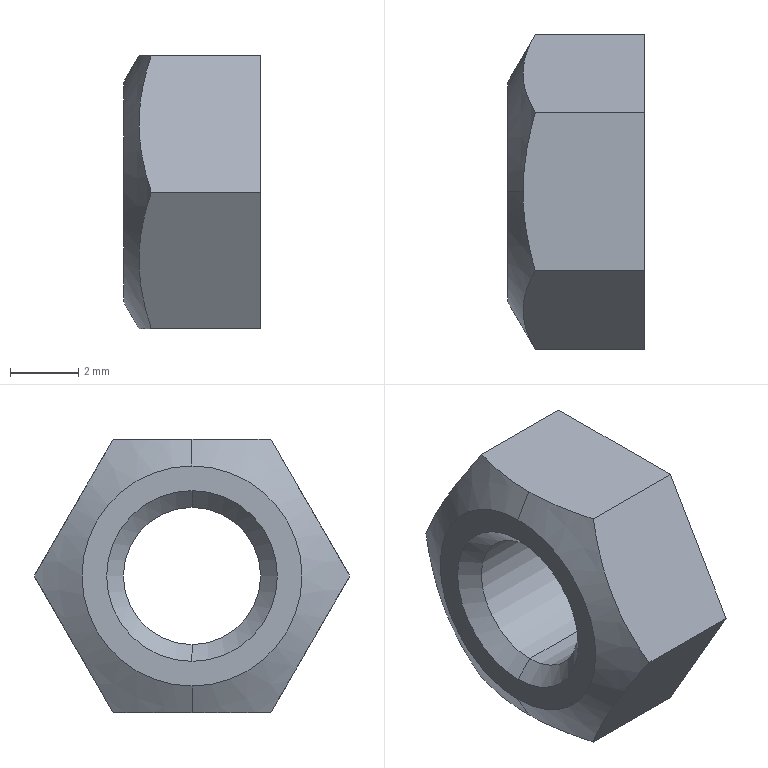Part | SolidWorks | features ICE 1, RevCut 1, Revolution 1 | 1 solid | 16 faces | box 4 x 9.238 x 8 mm | volume 160.7 mm3 | plane 8 | cone 6 | cylinder 2 | commonest cylinder face diameters 4.017 x2
STEP:
#1=CARTESIAN_POINT('',(-0.4915,0.,-2.009));
#2=VERTEX_POINT('',#1);
#3=CARTESIAN_POINT('',(-0.4915,0.,2.009));
#4=VERTEX_POINT('',#3);
#5=CARTESIAN_POINT('',(-0.4915,0.,0.));
#6=DIRECTION('',(-1.,0.,0.));
#7=DIRECTION('',(0.,0.,1.));
#8=AXIS2_PLACEMENT_3D('',#5,#6,#7);
#9=CIRCLE('',#8,2.009);
#10=EDGE_CURVE('',#2,#4,#9,.T.);
#11=ORIENTED_EDGE('',*,*,#10,.T.);
#12=CARTESIAN_POINT('',(0.,0.,2.5));
#13=VERTEX_POINT('',#12);
#14=CARTESIAN_POINT('',(0.,0.,2.5));
#15=DIRECTION('',(0.7071,0.,0.7071));
#16=VECTOR('',#15,1000.);
#17=LINE('',#14,#16);
#18=EDGE_CURVE('',#4,#13,#17,.T.);
#19=ORIENTED_EDGE('',*,*,#18,.T.);
#20=CARTESIAN_POINT('',(0.,0.,-2.5));
#21=VERTEX_POINT('',#20);
#22=CARTESIAN_POINT('',(0.,0.,0.));
#23=DIRECTION('',(-1.,0.,0.));
#24=DIRECTION('',(0.,0.,1.));
#25=AXIS2_PLACEMENT_3D('',#22,#23,#24);
#26=CIRCLE('',#25,2.5);
#27=EDGE_CURVE('',#21,#13,#26,.T.);
#28=ORIENTED_EDGE('',*,*,#27,.F.);
#29=CARTESIAN_POINT('',(0.,0.,-2.5));
#30=DIRECTION('',(0.7071,0.,-0.7071));
#31=VECTOR('',#30,1000.);
#32=LINE('',#29,#31);
#33=EDGE_CURVE('',#2,#21,#32,.T.);
#34=ORIENTED_EDGE('',*,*,#33,.F.);
#35=EDGE_LOOP('',(#11,#19,#28,#34));
#36=FACE_OUTER_BOUND('',#35,.T.);
#37=CARTESIAN_POINT('',(0.,0.,0.));
#38=DIRECTION('',(1.,0.,0.));
#39=DIRECTION('',(0.,0.,-1.));
#40=AXIS2_PLACEMENT_3D('',#37,#38,#39);
#41=CONICAL_SURFACE('',#40,2.5,0.7854);
#42=ADVANCED_FACE('',(#36),#41,.F.);
#43=ORIENTED_EDGE('',*,*,#10,.F.);
#44=CARTESIAN_POINT('',(-3.509,0.,-2.009));
#45=VERTEX_POINT('',#44);
#46=CARTESIAN_POINT('',(0.,0.,-2.009));
#47=DIRECTION('',(-1.,0.,0.));
#48=VECTOR('',#47,1000.);
#49=LINE('',#46,#48);
#50=EDGE_CURVE('',#2,#45,#49,.T.);
#51=ORIENTED_EDGE('',*,*,#50,.T.);
#52=CARTESIAN_POINT('',(-3.509,0.,2.009));
#53=VERTEX_POINT('',#52);
#54=CARTESIAN_POINT('',(-3.509,0.,0.));
#55=DIRECTION('',(-1.,0.,0.));
#56=DIRECTION('',(0.,0.,1.));
#57=AXIS2_PLACEMENT_3D('',#54,#55,#56);
#58=CIRCLE('',#57,2.009);
#59=EDGE_CURVE('',#45,#53,#58,.T.);
#60=ORIENTED_EDGE('',*,*,#59,.T.);
#61=CARTESIAN_POINT('',(0.,0.,2.009));
#62=DIRECTION('',(-1.,0.,0.));
#63=VECTOR('',#62,1000.);
#64=LINE('',#61,#63);
#65=EDGE_CURVE('',#4,#53,#64,.T.);
#66=ORIENTED_EDGE('',*,*,#65,.F.);
#67=EDGE_LOOP('',(#43,#51,#60,#66));
#68=FACE_OUTER_BOUND('',#67,.T.);
#69=CARTESIAN_POINT('',(0.,0.,0.));
#70=DIRECTION('',(-1.,0.,0.));
#71=DIRECTION('',(0.,0.,1.));
#72=AXIS2_PLACEMENT_3D('',#69,#70,#71);
#73=CYLINDRICAL_SURFACE('',#72,2.009);
#74=ADVANCED_FACE('',(#68),#73,.F.);
#75=ORIENTED_EDGE('',*,*,#59,.F.);
#76=CARTESIAN_POINT('',(-4.,0.,-2.5));
#77=VERTEX_POINT('',#76);
#78=CARTESIAN_POINT('',(-3.509,0.,-2.009));
#79=DIRECTION('',(-0.7071,0.,-0.7071));
#80=VECTOR('',#79,1000.);
#81=LINE('',#78,#80);
#82=EDGE_CURVE('',#45,#77,#81,.T.);
#83=ORIENTED_EDGE('',*,*,#82,.T.);
#84=CARTESIAN_POINT('',(-4.,0.,2.5));
#85=VERTEX_POINT('',#84);
#86=CARTESIAN_POINT('',(-4.,0.,0.));
#87=DIRECTION('',(-1.,0.,0.));
#88=DIRECTION('',(0.,0.,1.));
#89=AXIS2_PLACEMENT_3D('',#86,#87,#88);
#90=CIRCLE('',#89,2.5);
#91=EDGE_CURVE('',#77,#85,#90,.T.);
#92=ORIENTED_EDGE('',*,*,#91,.T.);
#93=CARTESIAN_POINT('',(-3.509,0.,2.009));
#94=DIRECTION('',(-0.7071,0.,0.7071));
#95=VECTOR('',#94,1000.);
#96=LINE('',#93,#95);
#97=EDGE_CURVE('',#53,#85,#96,.T.);
#98=ORIENTED_EDGE('',*,*,#97,.F.);
#99=EDGE_LOOP('',(#75,#83,#92,#98));
#100=FACE_OUTER_BOUND('',#99,.T.);
#101=CARTESIAN_POINT('',(-3.509,0.,0.));
#102=DIRECTION('',(-1.,0.,0.));
#103=DIRECTION('',(0.,0.,1.));
#104=AXIS2_PLACEMENT_3D('',#101,#102,#103);
#105=CONICAL_SURFACE('',#104,2.009,0.7854);
#106=ADVANCED_FACE('',(#100),#105,.F.);
#107=CARTESIAN_POINT('',(-4.,0.,3.22));
#108=VERTEX_POINT('',#107);
#109=CARTESIAN_POINT('',(-4.,0.,-3.22));
#110=VERTEX_POINT('',#109);
#111=CARTESIAN_POINT('',(-4.,0.,0.));
#112=DIRECTION('',(-1.,0.,0.));
#113=DIRECTION('',(0.,0.,1.));
#114=AXIS2_PLACEMENT_3D('',#111,#112,#113);
#115=CIRCLE('',#114,3.22);
#116=EDGE_CURVE('',#108,#110,#115,.T.);
#117=ORIENTED_EDGE('',*,*,#116,.F.);
#118=CARTESIAN_POINT('',(-3.55,0.,4.));
#119=VERTEX_POINT('',#118);
#120=CARTESIAN_POINT('',(-2.938,0.,5.06));
#121=DIRECTION('',(0.5,0.,0.866));
#122=VECTOR('',#121,1000.);
#123=LINE('',#120,#122);
#124=EDGE_CURVE('',#108,#119,#123,.T.);
#125=ORIENTED_EDGE('',*,*,#124,.T.);
#126=CARTESIAN_POINT('',(-3.192,2.309,4.));
#127=VERTEX_POINT('',#126);
#128=CARTESIAN_POINT('',(-3.192,2.309,4.));
#129=CARTESIAN_POINT('',(-3.3,1.936,4.));
#130=CARTESIAN_POINT('',(-3.39,1.558,4.));
#131=CARTESIAN_POINT('',(-3.515,0.7861,4.));
#132=CARTESIAN_POINT('',(-3.55,0.3904,4.));
#133=CARTESIAN_POINT('',(-3.55,0.,4.));
#134=B_SPLINE_CURVE_WITH_KNOTS('',3,(#128,#129,#130,#131,#132,#133),.UNSPECIFIED.,.F.,.F.,(4,2,4),(0.01066,0.01183,0.01301),.UNSPECIFIED.);
#135=EDGE_CURVE('',#127,#119,#134,.T.);
#136=ORIENTED_EDGE('',*,*,#135,.F.);
#137=CARTESIAN_POINT('',(-3.192,4.619,0.));
#138=VERTEX_POINT('',#137);
#139=CARTESIAN_POINT('',(-3.192,4.619,0.));
#140=CARTESIAN_POINT('',(-3.41,4.242,0.6531));
#141=CARTESIAN_POINT('',(-3.549,3.859,1.316));
#142=CARTESIAN_POINT('',(-3.55,3.27,2.336));
#143=CARTESIAN_POINT('',(-3.516,3.074,2.676));
#144=CARTESIAN_POINT('',(-3.391,2.689,3.343));
#145=CARTESIAN_POINT('',(-3.301,2.498,3.673));
#146=CARTESIAN_POINT('',(-3.192,2.309,4.));
#147=B_SPLINE_CURVE_WITH_KNOTS('',3,(#139,#140,#141,#142,#143,#144,#145,#146),.UNSPECIFIED.,.F.,.F.,(4,2,2,4),(0.000000238,0.002333,0.003499,0.004665),.UNSPECIFIED.);
#148=EDGE_CURVE('',#138,#127,#147,.T.);
#149=ORIENTED_EDGE('',*,*,#148,.F.);
#150=CARTESIAN_POINT('',(-3.192,2.309,-4.));
#151=VERTEX_POINT('',#150);
#152=CARTESIAN_POINT('',(-3.192,2.309,-4.));
#153=CARTESIAN_POINT('',(-3.41,2.686,-3.347));
#154=CARTESIAN_POINT('',(-3.549,3.069,-2.684));
#155=CARTESIAN_POINT('',(-3.55,3.658,-1.664));
#156=CARTESIAN_POINT('',(-3.516,3.854,-1.324));
#157=CARTESIAN_POINT('',(-3.391,4.24,-0.6567));
#158=CARTESIAN_POINT('',(-3.301,4.43,-0.327));
#159=CARTESIAN_POINT('',(-3.192,4.619,0.));
#160=B_SPLINE_CURVE_WITH_KNOTS('',3,(#152,#153,#154,#155,#156,#157,#158,#159),.UNSPECIFIED.,.F.,.F.,(4,2,2,4),(0.000000238,0.002333,0.003499,0.004665),.UNSPECIFIED.);
#161=EDGE_CURVE('',#151,#138,#160,.T.);
#162=ORIENTED_EDGE('',*,*,#161,.F.);
#163=CARTESIAN_POINT('',(-3.55,0.,-4.));
#164=VERTEX_POINT('',#163);
#165=CARTESIAN_POINT('',(-3.55,0.,-4.));
#166=CARTESIAN_POINT('',(-3.55,0.3904,-4.));
#167=CARTESIAN_POINT('',(-3.515,0.7861,-4.));
#168=CARTESIAN_POINT('',(-3.39,1.558,-4.));
#169=CARTESIAN_POINT('',(-3.3,1.936,-4.));
#170=CARTESIAN_POINT('',(-3.192,2.309,-4.));
#171=B_SPLINE_CURVE_WITH_KNOTS('',3,(#165,#166,#167,#168,#169,#170),.UNSPECIFIED.,.F.,.F.,(4,2,4),(0.006426,0.007595,0.008763),.UNSPECIFIED.);
#172=EDGE_CURVE('',#164,#151,#171,.T.);
#173=ORIENTED_EDGE('',*,*,#172,.F.);
#174=CARTESIAN_POINT('',(-2.938,0.,-5.06));
#175=DIRECTION('',(0.5,0.,-0.866));
#176=VECTOR('',#175,1000.);
#177=LINE('',#174,#176);
#178=EDGE_CURVE('',#110,#164,#177,.T.);
#179=ORIENTED_EDGE('',*,*,#178,.F.);
#180=EDGE_LOOP('',(#117,#125,#136,#149,#162,#173,#179));
#181=FACE_OUTER_BOUND('',#180,.T.);
#182=CARTESIAN_POINT('',(-2.938,0.,0.));
#183=DIRECTION('',(1.,0.,0.));
#184=DIRECTION('',(0.,0.,-1.));
#185=AXIS2_PLACEMENT_3D('',#182,#183,#184);
#186=CONICAL_SURFACE('',#185,5.06,1.047);
#187=ADVANCED_FACE('',(#181),#186,.T.);
#188=ORIENTED_EDGE('',*,*,#27,.T.);
#189=CARTESIAN_POINT('',(0.,0.,0.));
#190=DIRECTION('',(-1.,0.,0.));
#191=DIRECTION('',(0.,0.,1.));
#192=AXIS2_PLACEMENT_3D('',#189,#190,#191);
#193=CIRCLE('',#192,2.5);
#194=EDGE_CURVE('',#13,#21,#193,.T.);
#195=ORIENTED_EDGE('',*,*,#194,.T.);
#196=EDGE_LOOP('',(#188,#195));
#197=FACE_BOUND('',#196,.T.);
#198=CARTESIAN_POINT('',(0.,4.619,0.));
#199=VERTEX_POINT('',#198);
#200=CARTESIAN_POINT('',(0.,2.309,4.));
#201=VERTEX_POINT('',#200);
#202=CARTESIAN_POINT('',(0.,4.619,0.));
#203=DIRECTION('',(0.,-0.5,0.866));
#204=VECTOR('',#203,1000.);
#205=LINE('',#202,#204);
#206=EDGE_CURVE('',#199,#201,#205,.T.);
#207=ORIENTED_EDGE('',*,*,#206,.T.);
#208=CARTESIAN_POINT('',(0.,-2.309,4.));
#209=VERTEX_POINT('',#208);
#210=CARTESIAN_POINT('',(0.,2.309,4.));
#211=DIRECTION('',(0.,-1.,0.));
#212=VECTOR('',#211,1000.);
#213=LINE('',#210,#212);
#214=EDGE_CURVE('',#201,#209,#213,.T.);
#215=ORIENTED_EDGE('',*,*,#214,.T.);
#216=CARTESIAN_POINT('',(0.,-4.619,0.));
#217=VERTEX_POINT('',#216);
#218=CARTESIAN_POINT('',(0.,-2.309,4.));
#219=DIRECTION('',(0.,-0.5,-0.866));
#220=VECTOR('',#219,1000.);
#221=LINE('',#218,#220);
#222=EDGE_CURVE('',#209,#217,#221,.T.);
#223=ORIENTED_EDGE('',*,*,#222,.T.);
#224=CARTESIAN_POINT('',(0.,-2.309,-4.));
#225=VERTEX_POINT('',#224);
#226=CARTESIAN_POINT('',(0.,-4.619,0.));
#227=DIRECTION('',(0.,0.5,-0.866));
#228=VECTOR('',#227,1000.);
#229=LINE('',#226,#228);
#230=EDGE_CURVE('',#217,#225,#229,.T.);
#231=ORIENTED_EDGE('',*,*,#230,.T.);
#232=CARTESIAN_POINT('',(0.,2.309,-4.));
#233=VERTEX_POINT('',#232);
#234=CARTESIAN_POINT('',(0.,-2.309,-4.));
#235=DIRECTION('',(0.,1.,0.));
#236=VECTOR('',#235,1000.);
#237=LINE('',#234,#236);
#238=EDGE_CURVE('',#225,#233,#237,.T.);
#239=ORIENTED_EDGE('',*,*,#238,.T.);
#240=CARTESIAN_POINT('',(0.,2.309,-4.));
#241=DIRECTION('',(0.,0.5,0.866));
#242=VECTOR('',#241,1000.);
#243=LINE('',#240,#242);
#244=EDGE_CURVE('',#233,#199,#243,.T.);
#245=ORIENTED_EDGE('',*,*,#244,.T.);
#246=EDGE_LOOP('',(#207,#215,#223,#231,#239,#245));
#247=FACE_OUTER_BOUND('',#246,.T.);
#248=CARTESIAN_POINT('',(0.,5.06,0.));
#249=DIRECTION('',(-1.,0.,0.));
#250=DIRECTION('',(0.,0.,1.));
#251=AXIS2_PLACEMENT_3D('',#248,#249,#250);
#252=PLANE('',#251);
#253=ADVANCED_FACE('',(#197,#247),#252,.F.);
#254=ORIENTED_EDGE('',*,*,#124,.F.);
#255=CARTESIAN_POINT('',(-4.,0.,0.));
#256=DIRECTION('',(-1.,0.,0.));
#257=DIRECTION('',(0.,0.,1.));
#258=AXIS2_PLACEMENT_3D('',#255,#256,#257);
#259=CIRCLE('',#258,3.22);
#260=EDGE_CURVE('',#110,#108,#259,.T.);
#261=ORIENTED_EDGE('',*,*,#260,.F.);
#262=ORIENTED_EDGE('',*,*,#178,.T.);
#263=CARTESIAN_POINT('',(-3.192,-2.309,-4.));
#264=VERTEX_POINT('',#263);
#265=CARTESIAN_POINT('',(-3.192,-2.309,-4.));
#266=CARTESIAN_POINT('',(-3.301,-1.934,-4.));
#267=CARTESIAN_POINT('',(-3.392,-1.549,-4.));
#268=CARTESIAN_POINT('',(-3.516,-0.7779,-4.));
#269=CARTESIAN_POINT('',(-3.55,-0.3902,-4.));
#270=CARTESIAN_POINT('',(-3.55,0.,-4.));
#271=B_SPLINE_CURVE_WITH_KNOTS('',3,(#265,#266,#267,#268,#269,#270),.UNSPECIFIED.,.F.,.F.,(4,2,4),(0.00409,0.005258,0.006426),.UNSPECIFIED.);
#272=EDGE_CURVE('',#264,#164,#271,.T.);
#273=ORIENTED_EDGE('',*,*,#272,.F.);
#274=CARTESIAN_POINT('',(-3.192,-4.619,0.));
#275=VERTEX_POINT('',#274);
#276=CARTESIAN_POINT('',(-3.192,-4.619,0.));
#277=CARTESIAN_POINT('',(-3.41,-4.242,-0.6531));
#278=CARTESIAN_POINT('',(-3.549,-3.859,-1.316));
#279=CARTESIAN_POINT('',(-3.55,-3.27,-2.336));
#280=CARTESIAN_POINT('',(-3.516,-3.074,-2.676));
#281=CARTESIAN_POINT('',(-3.391,-2.689,-3.343));
#282=CARTESIAN_POINT('',(-3.301,-2.498,-3.673));
#283=CARTESIAN_POINT('',(-3.192,-2.309,-4.));
#284=B_SPLINE_CURVE_WITH_KNOTS('',3,(#276,#277,#278,#279,#280,#281,#282,#283),.UNSPECIFIED.,.F.,.F.,(4,2,2,4),(0.000000238,0.002333,0.003499,0.004665),.UNSPECIFIED.);
#285=EDGE_CURVE('',#275,#264,#284,.T.);
#286=ORIENTED_EDGE('',*,*,#285,.F.);
#287=CARTESIAN_POINT('',(-3.192,-2.309,4.));
#288=VERTEX_POINT('',#287);
#289=CARTESIAN_POINT('',(-3.192,-2.309,4.));
#290=CARTESIAN_POINT('',(-3.41,-2.686,3.347));
#291=CARTESIAN_POINT('',(-3.549,-3.069,2.684));
#292=CARTESIAN_POINT('',(-3.55,-3.658,1.664));
#293=CARTESIAN_POINT('',(-3.516,-3.854,1.324));
#294=CARTESIAN_POINT('',(-3.391,-4.24,0.6567));
#295=CARTESIAN_POINT('',(-3.301,-4.43,0.327));
#296=CARTESIAN_POINT('',(-3.192,-4.619,0.));
#297=B_SPLINE_CURVE_WITH_KNOTS('',3,(#289,#290,#291,#292,#293,#294,#295,#296),.UNSPECIFIED.,.F.,.F.,(4,2,2,4),(0.000000238,0.002333,0.003499,0.004665),.UNSPECIFIED.);
#298=EDGE_CURVE('',#288,#275,#297,.T.);
#299=ORIENTED_EDGE('',*,*,#298,.F.);
#300=CARTESIAN_POINT('',(-3.55,0.,4.));
#301=CARTESIAN_POINT('',(-3.55,-0.3902,4.));
#302=CARTESIAN_POINT('',(-3.516,-0.7779,4.));
#303=CARTESIAN_POINT('',(-3.392,-1.549,4.));
#304=CARTESIAN_POINT('',(-3.301,-1.934,4.));
#305=CARTESIAN_POINT('',(-3.192,-2.309,4.));
#306=B_SPLINE_CURVE_WITH_KNOTS('',3,(#300,#301,#302,#303,#304,#305),.UNSPECIFIED.,.F.,.F.,(4,2,4),(0.01301,0.01417,0.01534),.UNSPECIFIED.);
#307=EDGE_CURVE('',#119,#288,#306,.T.);
#308=ORIENTED_EDGE('',*,*,#307,.F.);
#309=EDGE_LOOP('',(#254,#261,#262,#273,#286,#299,#308));
#310=FACE_OUTER_BOUND('',#309,.T.);
#311=CARTESIAN_POINT('',(-2.938,0.,0.));
#312=DIRECTION('',(1.,0.,0.));
#313=DIRECTION('',(0.,0.,-1.));
#314=AXIS2_PLACEMENT_3D('',#311,#312,#313);
#315=CONICAL_SURFACE('',#314,5.06,1.047);
#316=ADVANCED_FACE('',(#310),#315,.T.);
#317=ORIENTED_EDGE('',*,*,#260,.T.);
#318=ORIENTED_EDGE('',*,*,#116,.T.);
#319=EDGE_LOOP('',(#317,#318));
#320=FACE_OUTER_BOUND('',#319,.T.);
#321=CARTESIAN_POINT('',(-4.,0.,0.));
#322=DIRECTION('',(-1.,0.,0.));
#323=DIRECTION('',(0.,0.,1.));
#324=AXIS2_PLACEMENT_3D('',#321,#322,#323);
#325=CIRCLE('',#324,2.5);
#326=EDGE_CURVE('',#85,#77,#325,.T.);
#327=ORIENTED_EDGE('',*,*,#326,.F.);
#328=ORIENTED_EDGE('',*,*,#91,.F.);
#329=EDGE_LOOP('',(#327,#328));
#330=FACE_BOUND('',#329,.T.);
#331=CARTESIAN_POINT('',(-4.,0.,0.));
#332=DIRECTION('',(1.,0.,0.));
#333=DIRECTION('',(0.,0.,-1.));
#334=AXIS2_PLACEMENT_3D('',#331,#332,#333);
#335=PLANE('',#334);
#336=ADVANCED_FACE('',(#320,#330),#335,.F.);
#337=ORIENTED_EDGE('',*,*,#82,.F.);
#338=CARTESIAN_POINT('',(-3.509,0.,0.));
#339=DIRECTION('',(-1.,0.,0.));
#340=DIRECTION('',(0.,0.,1.));
#341=AXIS2_PLACEMENT_3D('',#338,#339,#340);
#342=CIRCLE('',#341,2.009);
#343=EDGE_CURVE('',#53,#45,#342,.T.);
#344=ORIENTED_EDGE('',*,*,#343,.F.);
#345=ORIENTED_EDGE('',*,*,#97,.T.);
#346=ORIENTED_EDGE('',*,*,#326,.T.);
#347=EDGE_LOOP('',(#337,#344,#345,#346));
#348=FACE_OUTER_BOUND('',#347,.T.);
#349=CARTESIAN_POINT('',(-3.509,0.,0.));
#350=DIRECTION('',(-1.,0.,0.));
#351=DIRECTION('',(0.,0.,1.));
#352=AXIS2_PLACEMENT_3D('',#349,#350,#351);
#353=CONICAL_SURFACE('',#352,2.009,0.7854);
#354=ADVANCED_FACE('',(#348),#353,.F.);
#355=ORIENTED_EDGE('',*,*,#50,.F.);
#356=CARTESIAN_POINT('',(-0.4915,0.,0.));
#357=DIRECTION('',(-1.,0.,0.));
#358=DIRECTION('',(0.,0.,1.));
#359=AXIS2_PLACEMENT_3D('',#356,#357,#358);
#360=CIRCLE('',#359,2.009);
#361=EDGE_CURVE('',#4,#2,#360,.T.);
#362=ORIENTED_EDGE('',*,*,#361,.F.);
#363=ORIENTED_EDGE('',*,*,#65,.T.);
#364=ORIENTED_EDGE('',*,*,#343,.T.);
#365=EDGE_LOOP('',(#355,#362,#363,#364));
#366=FACE_OUTER_BOUND('',#365,.T.);
#367=CARTESIAN_POINT('',(0.,0.,0.));
#368=DIRECTION('',(-1.,0.,0.));
#369=DIRECTION('',(0.,0.,1.));
#370=AXIS2_PLACEMENT_3D('',#367,#368,#369);
#371=CYLINDRICAL_SURFACE('',#370,2.009);
#372=ADVANCED_FACE('',(#366),#371,.F.);
#373=ORIENTED_EDGE('',*,*,#18,.F.);
#374=ORIENTED_EDGE('',*,*,#361,.T.);
#375=ORIENTED_EDGE('',*,*,#33,.T.);
#376=ORIENTED_EDGE('',*,*,#194,.F.);
#377=EDGE_LOOP('',(#373,#374,#375,#376));
#378=FACE_OUTER_BOUND('',#377,.T.);
#379=CARTESIAN_POINT('',(0.,0.,0.));
#380=DIRECTION('',(1.,0.,0.));
#381=DIRECTION('',(0.,0.,-1.));
#382=AXIS2_PLACEMENT_3D('',#379,#380,#381);
#383=CONICAL_SURFACE('',#382,2.5,0.7854);
#384=ADVANCED_FACE('',(#378),#383,.F.);
#385=ORIENTED_EDGE('',*,*,#148,.T.);
#386=CARTESIAN_POINT('',(-4.,2.309,4.));
#387=DIRECTION('',(1.,0.,0.));
#388=VECTOR('',#387,1000.);
#389=LINE('',#386,#388);
#390=EDGE_CURVE('',#127,#201,#389,.T.);
#391=ORIENTED_EDGE('',*,*,#390,.T.);
#392=ORIENTED_EDGE('',*,*,#206,.F.);
#393=CARTESIAN_POINT('',(-4.,4.619,0.));
#394=DIRECTION('',(1.,0.,0.));
#395=VECTOR('',#394,1000.);
#396=LINE('',#393,#395);
#397=EDGE_CURVE('',#138,#199,#396,.T.);
#398=ORIENTED_EDGE('',*,*,#397,.F.);
#399=EDGE_LOOP('',(#385,#391,#392,#398));
#400=FACE_OUTER_BOUND('',#399,.T.);
#401=CARTESIAN_POINT('',(-4.,4.619,0.));
#402=DIRECTION('',(0.,0.866,0.5));
#403=DIRECTION('',(0.,-0.5,0.866));
#404=AXIS2_PLACEMENT_3D('',#401,#402,#403);
#405=PLANE('',#404);
#406=ADVANCED_FACE('',(#400),#405,.T.);
#407=ORIENTED_EDGE('',*,*,#161,.T.);
#408=ORIENTED_EDGE('',*,*,#397,.T.);
#409=ORIENTED_EDGE('',*,*,#244,.F.);
#410=CARTESIAN_POINT('',(-4.,2.309,-4.));
#411=DIRECTION('',(1.,0.,0.));
#412=VECTOR('',#411,1000.);
#413=LINE('',#410,#412);
#414=EDGE_CURVE('',#151,#233,#413,.T.);
#415=ORIENTED_EDGE('',*,*,#414,.F.);
#416=EDGE_LOOP('',(#407,#408,#409,#415));
#417=FACE_OUTER_BOUND('',#416,.T.);
#418=CARTESIAN_POINT('',(-4.,2.309,-4.));
#419=DIRECTION('',(0.,0.866,-0.5));
#420=DIRECTION('',(0.,0.5,0.866));
#421=AXIS2_PLACEMENT_3D('',#418,#419,#420);
#422=PLANE('',#421);
#423=ADVANCED_FACE('',(#417),#422,.T.);
#424=ORIENTED_EDGE('',*,*,#272,.T.);
#425=ORIENTED_EDGE('',*,*,#172,.T.);
#426=ORIENTED_EDGE('',*,*,#414,.T.);
#427=ORIENTED_EDGE('',*,*,#238,.F.);
#428=CARTESIAN_POINT('',(-4.,-2.309,-4.));
#429=DIRECTION('',(1.,0.,0.));
#430=VECTOR('',#429,1000.);
#431=LINE('',#428,#430);
#432=EDGE_CURVE('',#264,#225,#431,.T.);
#433=ORIENTED_EDGE('',*,*,#432,.F.);
#434=EDGE_LOOP('',(#424,#425,#426,#427,#433));
#435=FACE_OUTER_BOUND('',#434,.T.);
#436=CARTESIAN_POINT('',(-4.,-2.309,-4.));
#437=DIRECTION('',(0.,0.,-1.));
#438=DIRECTION('',(-1.,0.,0.));
#439=AXIS2_PLACEMENT_3D('',#436,#437,#438);
#440=PLANE('',#439);
#441=ADVANCED_FACE('',(#435),#440,.T.);
#442=ORIENTED_EDGE('',*,*,#285,.T.);
#443=ORIENTED_EDGE('',*,*,#432,.T.);
#444=ORIENTED_EDGE('',*,*,#230,.F.);
#445=CARTESIAN_POINT('',(-4.,-4.619,0.));
#446=DIRECTION('',(1.,0.,0.));
#447=VECTOR('',#446,1000.);
#448=LINE('',#445,#447);
#449=EDGE_CURVE('',#275,#217,#448,.T.);
#450=ORIENTED_EDGE('',*,*,#449,.F.);
#451=EDGE_LOOP('',(#442,#443,#444,#450));
#452=FACE_OUTER_BOUND('',#451,.T.);
#453=CARTESIAN_POINT('',(-4.,-4.619,0.));
#454=DIRECTION('',(0.,-0.866,-0.5));
#455=DIRECTION('',(0.,0.5,-0.866));
#456=AXIS2_PLACEMENT_3D('',#453,#454,#455);
#457=PLANE('',#456);
#458=ADVANCED_FACE('',(#452),#457,.T.);
#459=ORIENTED_EDGE('',*,*,#298,.T.);
#460=ORIENTED_EDGE('',*,*,#449,.T.);
#461=ORIENTED_EDGE('',*,*,#222,.F.);
#462=CARTESIAN_POINT('',(-4.,-2.309,4.));
#463=DIRECTION('',(1.,0.,0.));
#464=VECTOR('',#463,1000.);
#465=LINE('',#462,#464);
#466=EDGE_CURVE('',#288,#209,#465,.T.);
#467=ORIENTED_EDGE('',*,*,#466,.F.);
#468=EDGE_LOOP('',(#459,#460,#461,#467));
#469=FACE_OUTER_BOUND('',#468,.T.);
#470=CARTESIAN_POINT('',(-4.,-2.309,4.));
#471=DIRECTION('',(0.,-0.866,0.5));
#472=DIRECTION('',(0.,-0.5,-0.866));
#473=AXIS2_PLACEMENT_3D('',#470,#471,#472);
#474=PLANE('',#473);
#475=ADVANCED_FACE('',(#469),#474,.T.);
#476=ORIENTED_EDGE('',*,*,#135,.T.);
#477=ORIENTED_EDGE('',*,*,#307,.T.);
#478=ORIENTED_EDGE('',*,*,#466,.T.);
#479=ORIENTED_EDGE('',*,*,#214,.F.);
#480=ORIENTED_EDGE('',*,*,#390,.F.);
#481=EDGE_LOOP('',(#476,#477,#478,#479,#480));
#482=FACE_OUTER_BOUND('',#481,.T.);
#483=CARTESIAN_POINT('',(-4.,2.309,4.));
#484=DIRECTION('',(0.,0.,1.));
#485=DIRECTION('',(1.,0.,0.));
#486=AXIS2_PLACEMENT_3D('',#483,#484,#485);
#487=PLANE('',#486);
#488=ADVANCED_FACE('',(#482),#487,.T.);
#489=CLOSED_SHELL('',(#42,#74,#106,#187,#253,#316,#336,#354,#372,#384,#406,#423,#441,#458,#475,#488));
#490=MANIFOLD_SOLID_BREP('',#489);
#491=CARTESIAN_POINT('',(0.,0.,0.));
#492=DIRECTION('',(0.,0.,1.));
#493=DIRECTION('',(1.,0.,0.));
#494=AXIS2_PLACEMENT_3D('',#491,#492,#493);
#495=(LENGTH_UNIT()NAMED_UNIT(*)SI_UNIT(.MILLI.,.METRE.));
#496=UNCERTAINTY_MEASURE_WITH_UNIT(LENGTH_MEASURE(0.00001),#495,'','');
#497=(NAMED_UNIT(*)PLANE_ANGLE_UNIT()SI_UNIT($,.RADIAN.));
#498=(NAMED_UNIT(*)SI_UNIT($,.STERADIAN.)SOLID_ANGLE_UNIT());
#499=(GEOMETRIC_REPRESENTATION_CONTEXT(3)GLOBAL_UNCERTAINTY_ASSIGNED_CONTEXT((#496))GLOBAL_UNIT_ASSIGNED_CONTEXT((#495,#497,#498))REPRESENTATION_CONTEXT('',''));
#500=ADVANCED_BREP_SHAPE_REPRESENTATION('',(#490,#494),#499);